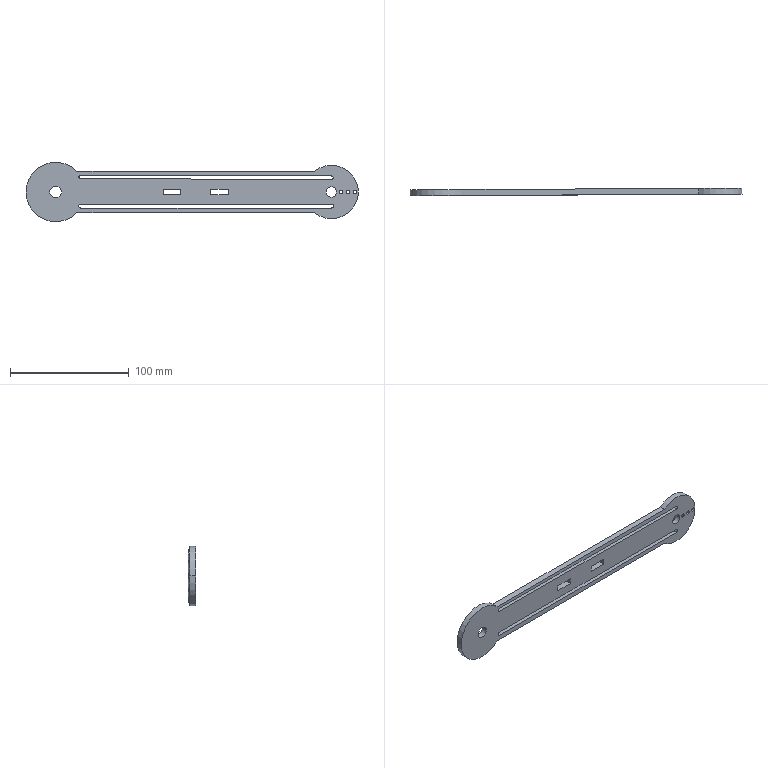Part | SolidWorks | features ICE 3, Extrusion 1 | 1 solid | 35 faces | box 279.515 x 6.264 x 50 mm | volume 42669 mm3 | cylinder 19 | plane 16 | commonest cylinder face diameters 3 x9 3.268 x3 8.5 x2 10 x2 50 x2 45 x1
STEP:
#1=CARTESIAN_POINT('',(-111.192,316.68,396.082));
#2=VERTEX_POINT('',#1);
#3=CARTESIAN_POINT('',(-112.826,316.673,394.448));
#4=VERTEX_POINT('',#3);
#5=CARTESIAN_POINT('',(-111.192,316.68,394.448));
#6=DIRECTION('',(0.004524,-1.,0.));
#7=DIRECTION('',(1.,0.004524,0.));
#8=AXIS2_PLACEMENT_3D('',#5,#6,#7);
#9=CIRCLE('',#8,1.634);
#10=EDGE_CURVE('',#2,#4,#9,.T.);
#11=ORIENTED_EDGE('',*,*,#10,.T.);
#12=CARTESIAN_POINT('',(-112.848,321.673,394.448));
#13=VERTEX_POINT('',#12);
#14=CARTESIAN_POINT('',(-112.803,311.673,394.448));
#15=DIRECTION('',(-0.004524,1.,0.));
#16=VECTOR('',#15,1000.);
#17=LINE('',#14,#16);
#18=EDGE_CURVE('',#4,#13,#17,.T.);
#19=ORIENTED_EDGE('',*,*,#18,.T.);
#20=CARTESIAN_POINT('',(-111.214,321.68,396.082));
#21=VERTEX_POINT('',#20);
#22=CARTESIAN_POINT('',(-111.214,321.68,394.448));
#23=DIRECTION('',(-0.004524,1.,0.));
#24=DIRECTION('',(-1.,-0.004524,0.));
#25=AXIS2_PLACEMENT_3D('',#22,#23,#24);
#26=CIRCLE('',#25,1.634);
#27=EDGE_CURVE('',#13,#21,#26,.T.);
#28=ORIENTED_EDGE('',*,*,#27,.T.);
#29=CARTESIAN_POINT('',(-111.169,311.68,396.082));
#30=DIRECTION('',(-0.004524,1.,0.));
#31=VECTOR('',#30,1000.);
#32=LINE('',#29,#31);
#33=EDGE_CURVE('',#2,#21,#32,.T.);
#34=ORIENTED_EDGE('',*,*,#33,.F.);
#35=EDGE_LOOP('',(#11,#19,#28,#34));
#36=FACE_OUTER_BOUND('',#35,.T.);
#37=CARTESIAN_POINT('',(-111.169,311.68,394.448));
#38=DIRECTION('',(-0.004524,1.,0.));
#39=DIRECTION('',(-1.,-0.004524,0.));
#40=AXIS2_PLACEMENT_3D('',#37,#38,#39);
#41=CYLINDRICAL_SURFACE('',#40,1.634);
#42=ADVANCED_FACE('',(#36),#41,.F.);
#43=CARTESIAN_POINT('',(-111.186,316.68,420.593));
#44=VERTEX_POINT('',#43);
#45=CARTESIAN_POINT('',(-112.692,316.673,419.093));
#46=VERTEX_POINT('',#45);
#47=CARTESIAN_POINT('',(-111.192,316.68,419.093));
#48=DIRECTION('',(0.004524,-1.,0.));
#49=DIRECTION('',(1.,0.004524,0.));
#50=AXIS2_PLACEMENT_3D('',#47,#48,#49);
#51=CIRCLE('',#50,1.5);
#52=EDGE_CURVE('',#44,#46,#51,.T.);
#53=ORIENTED_EDGE('',*,*,#52,.T.);
#54=CARTESIAN_POINT('',(-112.714,321.673,419.093));
#55=VERTEX_POINT('',#54);
#56=CARTESIAN_POINT('',(-112.669,311.673,419.093));
#57=DIRECTION('',(-0.004524,1.,0.));
#58=VECTOR('',#57,1000.);
#59=LINE('',#56,#58);
#60=EDGE_CURVE('',#46,#55,#59,.T.);
#61=ORIENTED_EDGE('',*,*,#60,.T.);
#62=CARTESIAN_POINT('',(-111.209,321.68,420.593));
#63=VERTEX_POINT('',#62);
#64=CARTESIAN_POINT('',(-111.214,321.68,419.093));
#65=DIRECTION('',(-0.004524,1.,0.));
#66=DIRECTION('',(1.,0.004524,0.));
#67=AXIS2_PLACEMENT_3D('',#64,#65,#66);
#68=CIRCLE('',#67,1.5);
#69=EDGE_CURVE('',#55,#63,#68,.T.);
#70=ORIENTED_EDGE('',*,*,#69,.T.);
#71=CARTESIAN_POINT('',(-111.164,311.68,420.593));
#72=DIRECTION('',(-0.004524,1.,0.));
#73=VECTOR('',#72,1000.);
#74=LINE('',#71,#73);
#75=EDGE_CURVE('',#44,#63,#74,.T.);
#76=ORIENTED_EDGE('',*,*,#75,.F.);
#77=EDGE_LOOP('',(#53,#61,#70,#76));
#78=FACE_OUTER_BOUND('',#77,.T.);
#79=CARTESIAN_POINT('',(-111.169,311.68,419.093));
#80=DIRECTION('',(-0.004524,1.,0.));
#81=DIRECTION('',(-1.,-0.004524,0.));
#82=AXIS2_PLACEMENT_3D('',#79,#80,#81);
#83=CYLINDRICAL_SURFACE('',#82,1.5);
#84=ADVANCED_FACE('',(#78),#83,.F.);
#85=CARTESIAN_POINT('',(106.283,317.664,406.314));
#86=VERTEX_POINT('',#85);
#87=CARTESIAN_POINT('',(109.283,317.678,406.314));
#88=VERTEX_POINT('',#87);
#89=CARTESIAN_POINT('',(107.783,317.671,406.314));
#90=DIRECTION('',(0.004524,-1.,0.));
#91=DIRECTION('',(1.,0.004524,0.));
#92=AXIS2_PLACEMENT_3D('',#89,#90,#91);
#93=CIRCLE('',#92,1.5);
#94=EDGE_CURVE('',#86,#88,#93,.T.);
#95=ORIENTED_EDGE('',*,*,#94,.T.);
#96=CARTESIAN_POINT('',(109.261,322.678,406.314));
#97=VERTEX_POINT('',#96);
#98=CARTESIAN_POINT('',(109.306,312.678,406.314));
#99=DIRECTION('',(-0.004524,1.,0.));
#100=VECTOR('',#99,1000.);
#101=LINE('',#98,#100);
#102=EDGE_CURVE('',#88,#97,#101,.T.);
#103=ORIENTED_EDGE('',*,*,#102,.T.);
#104=CARTESIAN_POINT('',(106.261,322.664,406.314));
#105=VERTEX_POINT('',#104);
#106=CARTESIAN_POINT('',(107.761,322.671,406.314));
#107=DIRECTION('',(-0.004524,1.,0.));
#108=DIRECTION('',(-1.,-0.004524,0.));
#109=AXIS2_PLACEMENT_3D('',#106,#107,#108);
#110=CIRCLE('',#109,1.5);
#111=EDGE_CURVE('',#97,#105,#110,.T.);
#112=ORIENTED_EDGE('',*,*,#111,.T.);
#113=CARTESIAN_POINT('',(106.306,312.664,406.314));
#114=DIRECTION('',(-0.004524,1.,0.));
#115=VECTOR('',#114,1000.);
#116=LINE('',#113,#115);
#117=EDGE_CURVE('',#86,#105,#116,.T.);
#118=ORIENTED_EDGE('',*,*,#117,.F.);
#119=EDGE_LOOP('',(#95,#103,#112,#118));
#120=FACE_OUTER_BOUND('',#119,.T.);
#121=CARTESIAN_POINT('',(107.806,312.671,406.314));
#122=DIRECTION('',(-0.004524,1.,0.));
#123=DIRECTION('',(-1.,-0.004524,0.));
#124=AXIS2_PLACEMENT_3D('',#121,#122,#123);
#125=CYLINDRICAL_SURFACE('',#124,1.5);
#126=ADVANCED_FACE('',(#120),#125,.F.);
#127=CARTESIAN_POINT('',(112.283,317.691,406.314));
#128=VERTEX_POINT('',#127);
#129=CARTESIAN_POINT('',(115.283,317.705,406.314));
#130=VERTEX_POINT('',#129);
#131=CARTESIAN_POINT('',(113.783,317.698,406.314));
#132=DIRECTION('',(0.004524,-1.,0.));
#133=DIRECTION('',(1.,0.004524,0.));
#134=AXIS2_PLACEMENT_3D('',#131,#132,#133);
#135=CIRCLE('',#134,1.5);
#136=EDGE_CURVE('',#128,#130,#135,.T.);
#137=ORIENTED_EDGE('',*,*,#136,.T.);
#138=CARTESIAN_POINT('',(115.261,322.705,406.314));
#139=VERTEX_POINT('',#138);
#140=CARTESIAN_POINT('',(115.306,312.705,406.314));
#141=DIRECTION('',(-0.004524,1.,0.));
#142=VECTOR('',#141,1000.);
#143=LINE('',#140,#142);
#144=EDGE_CURVE('',#130,#139,#143,.T.);
#145=ORIENTED_EDGE('',*,*,#144,.T.);
#146=CARTESIAN_POINT('',(112.261,322.691,406.314));
#147=VERTEX_POINT('',#146);
#148=CARTESIAN_POINT('',(113.761,322.698,406.314));
#149=DIRECTION('',(-0.004524,1.,0.));
#150=DIRECTION('',(-1.,-0.004524,0.));
#151=AXIS2_PLACEMENT_3D('',#148,#149,#150);
#152=CIRCLE('',#151,1.5);
#153=EDGE_CURVE('',#139,#147,#152,.T.);
#154=ORIENTED_EDGE('',*,*,#153,.T.);
#155=CARTESIAN_POINT('',(112.306,312.691,406.314));
#156=DIRECTION('',(-0.004524,1.,0.));
#157=VECTOR('',#156,1000.);
#158=LINE('',#155,#157);
#159=EDGE_CURVE('',#128,#147,#158,.T.);
#160=ORIENTED_EDGE('',*,*,#159,.F.);
#161=EDGE_LOOP('',(#137,#145,#154,#160));
#162=FACE_OUTER_BOUND('',#161,.T.);
#163=CARTESIAN_POINT('',(113.806,312.698,406.314));
#164=DIRECTION('',(-0.004524,1.,0.));
#165=DIRECTION('',(-1.,-0.004524,0.));
#166=AXIS2_PLACEMENT_3D('',#163,#164,#165);
#167=CYLINDRICAL_SURFACE('',#166,1.5);
#168=ADVANCED_FACE('',(#162),#167,.F.);
#169=CARTESIAN_POINT('',(118.283,317.718,406.314));
#170=VERTEX_POINT('',#169);
#171=CARTESIAN_POINT('',(121.283,317.732,406.314));
#172=VERTEX_POINT('',#171);
#173=CARTESIAN_POINT('',(119.783,317.725,406.314));
#174=DIRECTION('',(0.004524,-1.,0.));
#175=DIRECTION('',(1.,0.004524,0.));
#176=AXIS2_PLACEMENT_3D('',#173,#174,#175);
#177=CIRCLE('',#176,1.5);
#178=EDGE_CURVE('',#170,#172,#177,.T.);
#179=ORIENTED_EDGE('',*,*,#178,.T.);
#180=CARTESIAN_POINT('',(121.261,322.732,406.314));
#181=VERTEX_POINT('',#180);
#182=CARTESIAN_POINT('',(121.306,312.732,406.314));
#183=DIRECTION('',(-0.004524,1.,0.));
#184=VECTOR('',#183,1000.);
#185=LINE('',#182,#184);
#186=EDGE_CURVE('',#172,#181,#185,.T.);
#187=ORIENTED_EDGE('',*,*,#186,.T.);
#188=CARTESIAN_POINT('',(118.261,322.718,406.314));
#189=VERTEX_POINT('',#188);
#190=CARTESIAN_POINT('',(119.761,322.725,406.314));
#191=DIRECTION('',(-0.004524,1.,0.));
#192=DIRECTION('',(-1.,-0.004524,0.));
#193=AXIS2_PLACEMENT_3D('',#190,#191,#192);
#194=CIRCLE('',#193,1.5);
#195=EDGE_CURVE('',#181,#189,#194,.T.);
#196=ORIENTED_EDGE('',*,*,#195,.T.);
#197=CARTESIAN_POINT('',(118.306,312.718,406.314));
#198=DIRECTION('',(-0.004524,1.,0.));
#199=VECTOR('',#198,1000.);
#200=LINE('',#197,#199);
#201=EDGE_CURVE('',#170,#189,#200,.T.);
#202=ORIENTED_EDGE('',*,*,#201,.F.);
#203=EDGE_LOOP('',(#179,#187,#196,#202));
#204=FACE_OUTER_BOUND('',#203,.T.);
#205=CARTESIAN_POINT('',(119.806,312.725,406.314));
#206=DIRECTION('',(-0.004524,1.,0.));
#207=DIRECTION('',(-1.,-0.004524,0.));
#208=AXIS2_PLACEMENT_3D('',#205,#206,#207);
#209=CYLINDRICAL_SURFACE('',#208,1.5);
#210=ADVANCED_FACE('',(#204),#209,.F.);
#211=CARTESIAN_POINT('',(-137.21,316.562,406.314));
#212=VERTEX_POINT('',#211);
#213=CARTESIAN_POINT('',(-127.21,316.608,406.314));
#214=VERTEX_POINT('',#213);
#215=CARTESIAN_POINT('',(-132.21,316.585,406.314));
#216=DIRECTION('',(0.004524,-1.,0.));
#217=DIRECTION('',(1.,0.004524,0.));
#218=AXIS2_PLACEMENT_3D('',#215,#216,#217);
#219=CIRCLE('',#218,5.);
#220=EDGE_CURVE('',#212,#214,#219,.T.);
#221=ORIENTED_EDGE('',*,*,#220,.T.);
#222=CARTESIAN_POINT('',(-127.233,321.608,406.314));
#223=VERTEX_POINT('',#222);
#224=CARTESIAN_POINT('',(-127.21,316.608,406.314));
#225=DIRECTION('',(-0.004524,1.,0.));
#226=VECTOR('',#225,1000.);
#227=LINE('',#224,#226);
#228=EDGE_CURVE('',#214,#223,#227,.T.);
#229=ORIENTED_EDGE('',*,*,#228,.T.);
#230=CARTESIAN_POINT('',(-137.232,321.562,406.314));
#231=VERTEX_POINT('',#230);
#232=CARTESIAN_POINT('',(-132.233,321.585,406.314));
#233=DIRECTION('',(0.004524,-1.,0.));
#234=DIRECTION('',(1.,0.004524,0.));
#235=AXIS2_PLACEMENT_3D('',#232,#233,#234);
#236=CIRCLE('',#235,5.);
#237=EDGE_CURVE('',#231,#223,#236,.T.);
#238=ORIENTED_EDGE('',*,*,#237,.F.);
#239=CARTESIAN_POINT('',(-137.21,316.562,406.314));
#240=DIRECTION('',(-0.004524,1.,0.));
#241=VECTOR('',#240,1000.);
#242=LINE('',#239,#241);
#243=EDGE_CURVE('',#212,#231,#242,.T.);
#244=ORIENTED_EDGE('',*,*,#243,.F.);
#245=EDGE_LOOP('',(#221,#229,#238,#244));
#246=FACE_OUTER_BOUND('',#245,.T.);
#247=CARTESIAN_POINT('',(-132.21,316.585,406.314));
#248=DIRECTION('',(-0.004524,1.,0.));
#249=DIRECTION('',(-1.,-0.004524,0.));
#250=AXIS2_PLACEMENT_3D('',#247,#248,#249);
#251=CYLINDRICAL_SURFACE('',#250,5.);
#252=ADVANCED_FACE('',(#246),#251,.F.);
#253=CARTESIAN_POINT('',(95.533,317.615,406.314));
#254=VERTEX_POINT('',#253);
#255=CARTESIAN_POINT('',(104.033,317.654,406.314));
#256=VERTEX_POINT('',#255);
#257=CARTESIAN_POINT('',(99.783,317.635,406.314));
#258=DIRECTION('',(0.004524,-1.,0.));
#259=DIRECTION('',(1.,0.004524,0.));
#260=AXIS2_PLACEMENT_3D('',#257,#258,#259);
#261=CIRCLE('',#260,4.25);
#262=EDGE_CURVE('',#254,#256,#261,.T.);
#263=ORIENTED_EDGE('',*,*,#262,.T.);
#264=CARTESIAN_POINT('',(104.011,322.654,406.314));
#265=VERTEX_POINT('',#264);
#266=CARTESIAN_POINT('',(104.033,317.654,406.314));
#267=DIRECTION('',(-0.004524,1.,0.));
#268=VECTOR('',#267,1000.);
#269=LINE('',#266,#268);
#270=EDGE_CURVE('',#256,#265,#269,.T.);
#271=ORIENTED_EDGE('',*,*,#270,.T.);
#272=CARTESIAN_POINT('',(95.511,322.615,406.314));
#273=VERTEX_POINT('',#272);
#274=CARTESIAN_POINT('',(99.761,322.635,406.314));
#275=DIRECTION('',(0.004524,-1.,0.));
#276=DIRECTION('',(1.,0.004524,0.));
#277=AXIS2_PLACEMENT_3D('',#274,#275,#276);
#278=CIRCLE('',#277,4.25);
#279=EDGE_CURVE('',#273,#265,#278,.T.);
#280=ORIENTED_EDGE('',*,*,#279,.F.);
#281=CARTESIAN_POINT('',(95.533,317.615,406.314));
#282=DIRECTION('',(-0.004524,1.,0.));
#283=VECTOR('',#282,1000.);
#284=LINE('',#281,#283);
#285=EDGE_CURVE('',#254,#273,#284,.T.);
#286=ORIENTED_EDGE('',*,*,#285,.F.);
#287=EDGE_LOOP('',(#263,#271,#280,#286));
#288=FACE_OUTER_BOUND('',#287,.T.);
#289=CARTESIAN_POINT('',(99.783,317.635,406.314));
#290=DIRECTION('',(-0.004524,1.,0.));
#291=DIRECTION('',(-1.,-0.004524,0.));
#292=AXIS2_PLACEMENT_3D('',#289,#290,#291);
#293=CYLINDRICAL_SURFACE('',#292,4.25);
#294=ADVANCED_FACE('',(#288),#293,.F.);
#295=CARTESIAN_POINT('',(-157.21,316.472,406.314));
#296=VERTEX_POINT('',#295);
#297=CARTESIAN_POINT('',(-114.357,316.666,388.814));
#298=VERTEX_POINT('',#297);
#299=CARTESIAN_POINT('',(-132.21,316.585,406.314));
#300=DIRECTION('',(0.004524,-1.,0.));
#301=DIRECTION('',(1.,0.004524,0.));
#302=AXIS2_PLACEMENT_3D('',#299,#300,#301);
#303=CIRCLE('',#302,25.);
#304=EDGE_CURVE('',#296,#298,#303,.T.);
#305=ORIENTED_EDGE('',*,*,#304,.F.);
#306=CARTESIAN_POINT('',(-157.232,321.472,406.314));
#307=VERTEX_POINT('',#306);
#308=CARTESIAN_POINT('',(-157.21,316.472,406.314));
#309=DIRECTION('',(-0.004524,1.,0.));
#310=VECTOR('',#309,1000.);
#311=LINE('',#308,#310);
#312=EDGE_CURVE('',#296,#307,#311,.T.);
#313=ORIENTED_EDGE('',*,*,#312,.T.);
#314=CARTESIAN_POINT('',(-114.379,321.666,388.814));
#315=VERTEX_POINT('',#314);
#316=CARTESIAN_POINT('',(-132.233,321.585,406.314));
#317=DIRECTION('',(0.004524,-1.,0.));
#318=DIRECTION('',(1.,0.004524,0.));
#319=AXIS2_PLACEMENT_3D('',#316,#317,#318);
#320=CIRCLE('',#319,25.);
#321=EDGE_CURVE('',#307,#315,#320,.T.);
#322=ORIENTED_EDGE('',*,*,#321,.T.);
#323=CARTESIAN_POINT('',(-114.357,316.666,388.814));
#324=DIRECTION('',(-0.004524,1.,0.));
#325=VECTOR('',#324,1000.);
#326=LINE('',#323,#325);
#327=EDGE_CURVE('',#298,#315,#326,.T.);
#328=ORIENTED_EDGE('',*,*,#327,.F.);
#329=EDGE_LOOP('',(#305,#313,#322,#328));
#330=FACE_OUTER_BOUND('',#329,.T.);
#331=CARTESIAN_POINT('',(-132.21,316.585,406.314));
#332=DIRECTION('',(-0.004524,1.,0.));
#333=DIRECTION('',(-1.,-0.004524,0.));
#334=AXIS2_PLACEMENT_3D('',#331,#332,#333);
#335=CYLINDRICAL_SURFACE('',#334,25.);
#336=ADVANCED_FACE('',(#330),#335,.T.);
#337=CARTESIAN_POINT('',(-41.857,316.994,408.814));
#338=VERTEX_POINT('',#337);
#339=CARTESIAN_POINT('',(-41.857,316.994,403.814));
#340=VERTEX_POINT('',#339);
#341=CARTESIAN_POINT('',(-41.857,316.994,406.314));
#342=DIRECTION('',(0.,0.,-1.));
#343=VECTOR('',#342,1000.);
#344=LINE('',#341,#343);
#345=EDGE_CURVE('',#338,#340,#344,.T.);
#346=ORIENTED_EDGE('',*,*,#345,.F.);
#347=CARTESIAN_POINT('',(-26.857,317.062,408.814));
#348=VERTEX_POINT('',#347);
#349=CARTESIAN_POINT('',(99.783,317.635,408.814));
#350=DIRECTION('',(-1.,-0.004524,0.));
#351=VECTOR('',#350,1000.);
#352=LINE('',#349,#351);
#353=EDGE_CURVE('',#348,#338,#352,.T.);
#354=ORIENTED_EDGE('',*,*,#353,.F.);
#355=CARTESIAN_POINT('',(-26.857,317.062,403.814));
#356=VERTEX_POINT('',#355);
#357=CARTESIAN_POINT('',(-26.857,317.062,406.314));
#358=DIRECTION('',(0.,0.,1.));
#359=VECTOR('',#358,1000.);
#360=LINE('',#357,#359);
#361=EDGE_CURVE('',#356,#348,#360,.T.);
#362=ORIENTED_EDGE('',*,*,#361,.F.);
#363=CARTESIAN_POINT('',(99.783,317.635,403.814));
#364=DIRECTION('',(1.,0.004524,0.));
#365=VECTOR('',#364,1000.);
#366=LINE('',#363,#365);
#367=EDGE_CURVE('',#340,#356,#366,.T.);
#368=ORIENTED_EDGE('',*,*,#367,.F.);
#369=EDGE_LOOP('',(#346,#354,#362,#368));
#370=FACE_BOUND('',#369,.T.);
#371=CARTESIAN_POINT('',(-1.858,317.175,408.814));
#372=VERTEX_POINT('',#371);
#373=CARTESIAN_POINT('',(-1.858,317.175,403.814));
#374=VERTEX_POINT('',#373);
#375=CARTESIAN_POINT('',(-1.858,317.175,406.314));
#376=DIRECTION('',(0.,0.,-1.));
#377=VECTOR('',#376,1000.);
#378=LINE('',#375,#377);
#379=EDGE_CURVE('',#372,#374,#378,.T.);
#380=ORIENTED_EDGE('',*,*,#379,.F.);
#381=CARTESIAN_POINT('',(13.142,317.243,408.814));
#382=VERTEX_POINT('',#381);
#383=CARTESIAN_POINT('',(99.783,317.635,408.814));
#384=DIRECTION('',(-1.,-0.004524,0.));
#385=VECTOR('',#384,1000.);
#386=LINE('',#383,#385);
#387=EDGE_CURVE('',#382,#372,#386,.T.);
#388=ORIENTED_EDGE('',*,*,#387,.F.);
#389=CARTESIAN_POINT('',(13.142,317.243,403.814));
#390=VERTEX_POINT('',#389);
#391=CARTESIAN_POINT('',(13.142,317.243,406.314));
#392=DIRECTION('',(0.,0.,1.));
#393=VECTOR('',#392,1000.);
#394=LINE('',#391,#393);
#395=EDGE_CURVE('',#390,#382,#394,.T.);
#396=ORIENTED_EDGE('',*,*,#395,.F.);
#397=CARTESIAN_POINT('',(99.783,317.635,403.814));
#398=DIRECTION('',(1.,0.004524,0.));
#399=VECTOR('',#398,1000.);
#400=LINE('',#397,#399);
#401=EDGE_CURVE('',#374,#390,#400,.T.);
#402=ORIENTED_EDGE('',*,*,#401,.F.);
#403=EDGE_LOOP('',(#380,#388,#396,#402));
#404=FACE_BOUND('',#403,.T.);
#405=ORIENTED_EDGE('',*,*,#10,.F.);
#406=CARTESIAN_POINT('',(99.783,317.635,396.082));
#407=VERTEX_POINT('',#406);
#408=CARTESIAN_POINT('',(99.783,317.635,396.082));
#409=DIRECTION('',(-1.,-0.004524,0.));
#410=VECTOR('',#409,1000.);
#411=LINE('',#408,#410);
#412=EDGE_CURVE('',#407,#2,#411,.T.);
#413=ORIENTED_EDGE('',*,*,#412,.F.);
#414=CARTESIAN_POINT('',(99.783,317.635,392.814));
#415=VERTEX_POINT('',#414);
#416=CARTESIAN_POINT('',(99.783,317.635,394.448));
#417=DIRECTION('',(0.004524,-1.,0.));
#418=DIRECTION('',(1.,0.004524,0.));
#419=AXIS2_PLACEMENT_3D('',#416,#417,#418);
#420=CIRCLE('',#419,1.634);
#421=EDGE_CURVE('',#415,#407,#420,.T.);
#422=ORIENTED_EDGE('',*,*,#421,.F.);
#423=CARTESIAN_POINT('',(-111.192,316.68,392.814));
#424=VERTEX_POINT('',#423);
#425=CARTESIAN_POINT('',(99.783,317.635,392.814));
#426=DIRECTION('',(1.,0.004524,0.));
#427=VECTOR('',#426,1000.);
#428=LINE('',#425,#427);
#429=EDGE_CURVE('',#424,#415,#428,.T.);
#430=ORIENTED_EDGE('',*,*,#429,.F.);
#431=CARTESIAN_POINT('',(-111.192,316.68,394.448));
#432=DIRECTION('',(0.004524,-1.,0.));
#433=DIRECTION('',(1.,0.004524,0.));
#434=AXIS2_PLACEMENT_3D('',#431,#432,#433);
#435=CIRCLE('',#434,1.634);
#436=EDGE_CURVE('',#4,#424,#435,.T.);
#437=ORIENTED_EDGE('',*,*,#436,.F.);
#438=EDGE_LOOP('',(#405,#413,#422,#430,#437));
#439=FACE_BOUND('',#438,.T.);
#440=ORIENTED_EDGE('',*,*,#52,.F.);
#441=CARTESIAN_POINT('',(99.783,317.635,419.814));
#442=VERTEX_POINT('',#441);
#443=CARTESIAN_POINT('',(99.833,317.635,419.814));
#444=DIRECTION('',(-1.,-0.004524,0.003693));
#445=VECTOR('',#444,1000.);
#446=LINE('',#443,#445);
#447=EDGE_CURVE('',#442,#44,#446,.T.);
#448=ORIENTED_EDGE('',*,*,#447,.F.);
#449=CARTESIAN_POINT('',(99.772,317.635,416.814));
#450=VERTEX_POINT('',#449);
#451=CARTESIAN_POINT('',(99.778,317.635,418.314));
#452=DIRECTION('',(0.004524,-1.,0.));
#453=DIRECTION('',(1.,0.004524,0.));
#454=AXIS2_PLACEMENT_3D('',#451,#452,#453);
#455=CIRCLE('',#454,1.5);
#456=EDGE_CURVE('',#450,#442,#455,.T.);
#457=ORIENTED_EDGE('',*,*,#456,.F.);
#458=CARTESIAN_POINT('',(-111.197,316.68,417.593));
#459=VERTEX_POINT('',#458);
#460=CARTESIAN_POINT('',(99.822,317.635,416.814));
#461=DIRECTION('',(1.,0.004524,-0.003693));
#462=VECTOR('',#461,1000.);
#463=LINE('',#460,#462);
#464=EDGE_CURVE('',#459,#450,#463,.T.);
#465=ORIENTED_EDGE('',*,*,#464,.F.);
#466=CARTESIAN_POINT('',(-111.192,316.68,419.093));
#467=DIRECTION('',(0.004524,-1.,0.));
#468=DIRECTION('',(1.,0.004524,0.));
#469=AXIS2_PLACEMENT_3D('',#466,#467,#468);
#470=CIRCLE('',#469,1.5);
#471=EDGE_CURVE('',#46,#459,#470,.T.);
#472=ORIENTED_EDGE('',*,*,#471,.F.);
#473=EDGE_LOOP('',(#440,#448,#457,#465,#472));
#474=FACE_BOUND('',#473,.T.);
#475=ORIENTED_EDGE('',*,*,#94,.F.);
#476=CARTESIAN_POINT('',(107.783,317.671,406.314));
#477=DIRECTION('',(0.004524,-1.,0.));
#478=DIRECTION('',(1.,0.004524,0.));
#479=AXIS2_PLACEMENT_3D('',#476,#477,#478);
#480=CIRCLE('',#479,1.5);
#481=EDGE_CURVE('',#88,#86,#480,.T.);
#482=ORIENTED_EDGE('',*,*,#481,.F.);
#483=EDGE_LOOP('',(#475,#482));
#484=FACE_BOUND('',#483,.T.);
#485=ORIENTED_EDGE('',*,*,#136,.F.);
#486=CARTESIAN_POINT('',(113.783,317.698,406.314));
#487=DIRECTION('',(0.004524,-1.,0.));
#488=DIRECTION('',(1.,0.004524,0.));
#489=AXIS2_PLACEMENT_3D('',#486,#487,#488);
#490=CIRCLE('',#489,1.5);
#491=EDGE_CURVE('',#130,#128,#490,.T.);
#492=ORIENTED_EDGE('',*,*,#491,.F.);
#493=EDGE_LOOP('',(#485,#492));
#494=FACE_BOUND('',#493,.T.);
#495=ORIENTED_EDGE('',*,*,#178,.F.);
#496=CARTESIAN_POINT('',(119.783,317.725,406.314));
#497=DIRECTION('',(0.004524,-1.,0.));
#498=DIRECTION('',(1.,0.004524,0.));
#499=AXIS2_PLACEMENT_3D('',#496,#497,#498);
#500=CIRCLE('',#499,1.5);
#501=EDGE_CURVE('',#172,#170,#500,.T.);
#502=ORIENTED_EDGE('',*,*,#501,.F.);
#503=EDGE_LOOP('',(#495,#502));
#504=FACE_BOUND('',#503,.T.);
#505=ORIENTED_EDGE('',*,*,#262,.F.);
#506=CARTESIAN_POINT('',(99.783,317.635,406.314));
#507=DIRECTION('',(0.004524,-1.,0.));
#508=DIRECTION('',(1.,0.004524,0.));
#509=AXIS2_PLACEMENT_3D('',#506,#507,#508);
#510=CIRCLE('',#509,4.25);
#511=EDGE_CURVE('',#256,#254,#510,.T.);
#512=ORIENTED_EDGE('',*,*,#511,.F.);
#513=EDGE_LOOP('',(#505,#512));
#514=FACE_BOUND('',#513,.T.);
#515=CARTESIAN_POINT('',(85.641,317.571,388.814));
#516=VERTEX_POINT('',#515);
#517=CARTESIAN_POINT('',(85.641,317.571,423.814));
#518=VERTEX_POINT('',#517);
#519=CARTESIAN_POINT('',(99.783,317.635,406.314));
#520=DIRECTION('',(0.004524,-1.,0.));
#521=DIRECTION('',(1.,0.004524,0.));
#522=AXIS2_PLACEMENT_3D('',#519,#520,#521);
#523=CIRCLE('',#522,22.5);
#524=EDGE_CURVE('',#516,#518,#523,.T.);
#525=ORIENTED_EDGE('',*,*,#524,.T.);
#526=CARTESIAN_POINT('',(-114.357,316.666,423.814));
#527=VERTEX_POINT('',#526);
#528=CARTESIAN_POINT('',(85.641,317.571,423.814));
#529=DIRECTION('',(-1.,-0.004524,0.));
#530=VECTOR('',#529,1000.);
#531=LINE('',#528,#530);
#532=EDGE_CURVE('',#518,#527,#531,.T.);
#533=ORIENTED_EDGE('',*,*,#532,.T.);
#534=CARTESIAN_POINT('',(-132.21,316.585,406.314));
#535=DIRECTION('',(0.004524,-1.,0.));
#536=DIRECTION('',(1.,0.004524,0.));
#537=AXIS2_PLACEMENT_3D('',#534,#535,#536);
#538=CIRCLE('',#537,25.);
#539=EDGE_CURVE('',#527,#296,#538,.T.);
#540=ORIENTED_EDGE('',*,*,#539,.T.);
#541=ORIENTED_EDGE('',*,*,#304,.T.);
#542=CARTESIAN_POINT('',(85.641,317.571,388.814));
#543=DIRECTION('',(1.,0.004524,0.));
#544=VECTOR('',#543,1000.);
#545=LINE('',#542,#544);
#546=EDGE_CURVE('',#298,#516,#545,.T.);
#547=ORIENTED_EDGE('',*,*,#546,.T.);
#548=EDGE_LOOP('',(#525,#533,#540,#541,#547));
#549=FACE_OUTER_BOUND('',#548,.T.);
#550=ORIENTED_EDGE('',*,*,#220,.F.);
#551=CARTESIAN_POINT('',(-132.21,316.585,406.314));
#552=DIRECTION('',(0.004524,-1.,0.));
#553=DIRECTION('',(1.,0.004524,0.));
#554=AXIS2_PLACEMENT_3D('',#551,#552,#553);
#555=CIRCLE('',#554,5.);
#556=EDGE_CURVE('',#214,#212,#555,.T.);
#557=ORIENTED_EDGE('',*,*,#556,.F.);
#558=EDGE_LOOP('',(#550,#557));
#559=FACE_BOUND('',#558,.T.);
#560=CARTESIAN_POINT('',(99.783,317.635,406.314));
#561=DIRECTION('',(0.004524,-1.,0.));
#562=DIRECTION('',(1.,0.004524,0.));
#563=AXIS2_PLACEMENT_3D('',#560,#561,#562);
#564=PLANE('',#563);
#565=ADVANCED_FACE('',(#370,#404,#439,#474,#484,#494,#504,#514,#549,#559),#564,.T.);
#566=CARTESIAN_POINT('',(-41.88,321.994,408.814));
#567=VERTEX_POINT('',#566);
#568=CARTESIAN_POINT('',(-26.88,322.062,408.814));
#569=VERTEX_POINT('',#568);
#570=CARTESIAN_POINT('',(-41.88,321.994,408.814));
#571=DIRECTION('',(1.,0.004524,0.));
#572=VECTOR('',#571,1000.);
#573=LINE('',#570,#572);
#574=EDGE_CURVE('',#567,#569,#573,.T.);
#575=ORIENTED_EDGE('',*,*,#574,.F.);
#576=CARTESIAN_POINT('',(-41.88,321.994,403.814));
#577=VERTEX_POINT('',#576);
#578=CARTESIAN_POINT('',(-41.88,321.994,408.814));
#579=DIRECTION('',(0.,0.,1.));
#580=VECTOR('',#579,1000.);
#581=LINE('',#578,#580);
#582=EDGE_CURVE('',#577,#567,#581,.T.);
#583=ORIENTED_EDGE('',*,*,#582,.F.);
#584=CARTESIAN_POINT('',(-26.88,322.062,403.814));
#585=VERTEX_POINT('',#584);
#586=CARTESIAN_POINT('',(-41.88,321.994,403.814));
#587=DIRECTION('',(-1.,-0.004524,0.));
#588=VECTOR('',#587,1000.);
#589=LINE('',#586,#588);
#590=EDGE_CURVE('',#585,#577,#589,.T.);
#591=ORIENTED_EDGE('',*,*,#590,.F.);
#592=CARTESIAN_POINT('',(-26.88,322.062,408.814));
#593=DIRECTION('',(0.,0.,-1.));
#594=VECTOR('',#593,1000.);
#595=LINE('',#592,#594);
#596=EDGE_CURVE('',#569,#585,#595,.T.);
#597=ORIENTED_EDGE('',*,*,#596,.F.);
#598=EDGE_LOOP('',(#575,#583,#591,#597));
#599=FACE_BOUND('',#598,.T.);
#600=CARTESIAN_POINT('',(-1.88,322.175,408.814));
#601=VERTEX_POINT('',#600);
#602=CARTESIAN_POINT('',(13.12,322.243,408.814));
#603=VERTEX_POINT('',#602);
#604=CARTESIAN_POINT('',(-1.88,322.175,408.814));
#605=DIRECTION('',(1.,0.004524,0.));
#606=VECTOR('',#605,1000.);
#607=LINE('',#604,#606);
#608=EDGE_CURVE('',#601,#603,#607,.T.);
#609=ORIENTED_EDGE('',*,*,#608,.F.);
#610=CARTESIAN_POINT('',(-1.88,322.175,403.814));
#611=VERTEX_POINT('',#610);
#612=CARTESIAN_POINT('',(-1.88,322.175,408.814));
#613=DIRECTION('',(0.,0.,1.));
#614=VECTOR('',#613,1000.);
#615=LINE('',#612,#614);
#616=EDGE_CURVE('',#611,#601,#615,.T.);
#617=ORIENTED_EDGE('',*,*,#616,.F.);
#618=CARTESIAN_POINT('',(13.12,322.243,403.814));
#619=VERTEX_POINT('',#618);
#620=CARTESIAN_POINT('',(-1.88,322.175,403.814));
#621=DIRECTION('',(-1.,-0.004524,0.));
#622=VECTOR('',#621,1000.);
#623=LINE('',#620,#622);
#624=EDGE_CURVE('',#619,#611,#623,.T.);
#625=ORIENTED_EDGE('',*,*,#624,.F.);
#626=CARTESIAN_POINT('',(13.12,322.243,408.814));
#627=DIRECTION('',(0.,0.,-1.));
#628=VECTOR('',#627,1000.);
#629=LINE('',#626,#628);
#630=EDGE_CURVE('',#603,#619,#629,.T.);
#631=ORIENTED_EDGE('',*,*,#630,.F.);
#632=EDGE_LOOP('',(#609,#617,#625,#631));
#633=FACE_BOUND('',#632,.T.);
#634=CARTESIAN_POINT('',(99.761,322.635,396.082));
#635=VERTEX_POINT('',#634);
#636=CARTESIAN_POINT('',(-111.214,321.68,396.082));
#637=DIRECTION('',(1.,0.004524,0.));
#638=VECTOR('',#637,1000.);
#639=LINE('',#636,#638);
#640=EDGE_CURVE('',#21,#635,#639,.T.);
#641=ORIENTED_EDGE('',*,*,#640,.F.);
#642=ORIENTED_EDGE('',*,*,#27,.F.);
#643=CARTESIAN_POINT('',(-111.214,321.68,392.814));
#644=VERTEX_POINT('',#643);
#645=CARTESIAN_POINT('',(-111.214,321.68,394.448));
#646=DIRECTION('',(-0.004524,1.,0.));
#647=DIRECTION('',(-1.,-0.004524,0.));
#648=AXIS2_PLACEMENT_3D('',#645,#646,#647);
#649=CIRCLE('',#648,1.634);
#650=EDGE_CURVE('',#644,#13,#649,.T.);
#651=ORIENTED_EDGE('',*,*,#650,.F.);
#652=CARTESIAN_POINT('',(99.761,322.635,392.814));
#653=VERTEX_POINT('',#652);
#654=CARTESIAN_POINT('',(-111.214,321.68,392.814));
#655=DIRECTION('',(-1.,-0.004524,0.));
#656=VECTOR('',#655,1000.);
#657=LINE('',#654,#656);
#658=EDGE_CURVE('',#653,#644,#657,.T.);
#659=ORIENTED_EDGE('',*,*,#658,.F.);
#660=CARTESIAN_POINT('',(99.761,322.635,394.448));
#661=DIRECTION('',(-0.004524,1.,0.));
#662=DIRECTION('',(-1.,-0.004524,0.));
#663=AXIS2_PLACEMENT_3D('',#660,#661,#662);
#664=CIRCLE('',#663,1.634);
#665=EDGE_CURVE('',#635,#653,#664,.T.);
#666=ORIENTED_EDGE('',*,*,#665,.F.);
#667=EDGE_LOOP('',(#641,#642,#651,#659,#666));
#668=FACE_BOUND('',#667,.T.);
#669=CARTESIAN_POINT('',(99.761,322.635,419.814));
#670=VERTEX_POINT('',#669);
#671=CARTESIAN_POINT('',(-111.209,321.68,420.593));
#672=DIRECTION('',(1.,0.004524,-0.003693));
#673=VECTOR('',#672,1000.);
#674=LINE('',#671,#673);
#675=EDGE_CURVE('',#63,#670,#674,.T.);
#676=ORIENTED_EDGE('',*,*,#675,.F.);
#677=ORIENTED_EDGE('',*,*,#69,.F.);
#678=CARTESIAN_POINT('',(-111.22,321.68,417.593));
#679=VERTEX_POINT('',#678);
#680=CARTESIAN_POINT('',(-111.214,321.68,419.093));
#681=DIRECTION('',(-0.004524,1.,0.));
#682=DIRECTION('',(1.,0.004524,0.));
#683=AXIS2_PLACEMENT_3D('',#680,#681,#682);
#684=CIRCLE('',#683,1.5);
#685=EDGE_CURVE('',#679,#55,#684,.T.);
#686=ORIENTED_EDGE('',*,*,#685,.F.);
#687=CARTESIAN_POINT('',(99.75,322.635,416.814));
#688=VERTEX_POINT('',#687);
#689=CARTESIAN_POINT('',(-111.22,321.68,417.593));
#690=DIRECTION('',(-1.,-0.004524,0.003693));
#691=VECTOR('',#690,1000.);
#692=LINE('',#689,#691);
#693=EDGE_CURVE('',#688,#679,#692,.T.);
#694=ORIENTED_EDGE('',*,*,#693,.F.);
#695=CARTESIAN_POINT('',(99.755,322.635,418.314));
#696=DIRECTION('',(-0.004524,1.,0.));
#697=DIRECTION('',(1.,0.004524,0.));
#698=AXIS2_PLACEMENT_3D('',#695,#696,#697);
#699=CIRCLE('',#698,1.5);
#700=EDGE_CURVE('',#670,#688,#699,.T.);
#701=ORIENTED_EDGE('',*,*,#700,.F.);
#702=EDGE_LOOP('',(#676,#677,#686,#694,#701));
#703=FACE_BOUND('',#702,.T.);
#704=CARTESIAN_POINT('',(107.761,322.671,406.314));
#705=DIRECTION('',(-0.004524,1.,0.));
#706=DIRECTION('',(-1.,-0.004524,0.));
#707=AXIS2_PLACEMENT_3D('',#704,#705,#706);
#708=CIRCLE('',#707,1.5);
#709=EDGE_CURVE('',#105,#97,#708,.T.);
#710=ORIENTED_EDGE('',*,*,#709,.F.);
#711=ORIENTED_EDGE('',*,*,#111,.F.);
#712=EDGE_LOOP('',(#710,#711));
#713=FACE_BOUND('',#712,.T.);
#714=CARTESIAN_POINT('',(113.761,322.698,406.314));
#715=DIRECTION('',(-0.004524,1.,0.));
#716=DIRECTION('',(-1.,-0.004524,0.));
#717=AXIS2_PLACEMENT_3D('',#714,#715,#716);
#718=CIRCLE('',#717,1.5);
#719=EDGE_CURVE('',#147,#139,#718,.T.);
#720=ORIENTED_EDGE('',*,*,#719,.F.);
#721=ORIENTED_EDGE('',*,*,#153,.F.);
#722=EDGE_LOOP('',(#720,#721));
#723=FACE_BOUND('',#722,.T.);
#724=CARTESIAN_POINT('',(119.761,322.725,406.314));
#725=DIRECTION('',(-0.004524,1.,0.));
#726=DIRECTION('',(-1.,-0.004524,0.));
#727=AXIS2_PLACEMENT_3D('',#724,#725,#726);
#728=CIRCLE('',#727,1.5);
#729=EDGE_CURVE('',#189,#181,#728,.T.);
#730=ORIENTED_EDGE('',*,*,#729,.F.);
#731=ORIENTED_EDGE('',*,*,#195,.F.);
#732=EDGE_LOOP('',(#730,#731));
#733=FACE_BOUND('',#732,.T.);
#734=CARTESIAN_POINT('',(85.619,322.571,388.814));
#735=VERTEX_POINT('',#734);
#736=CARTESIAN_POINT('',(85.619,322.571,423.814));
#737=VERTEX_POINT('',#736);
#738=CARTESIAN_POINT('',(99.761,322.635,406.314));
#739=DIRECTION('',(0.004524,-1.,0.));
#740=DIRECTION('',(1.,0.004524,0.));
#741=AXIS2_PLACEMENT_3D('',#738,#739,#740);
#742=CIRCLE('',#741,22.5);
#743=EDGE_CURVE('',#735,#737,#742,.T.);
#744=ORIENTED_EDGE('',*,*,#743,.F.);
#745=CARTESIAN_POINT('',(85.619,322.571,388.814));
#746=DIRECTION('',(1.,0.004524,0.));
#747=VECTOR('',#746,1000.);
#748=LINE('',#745,#747);
#749=EDGE_CURVE('',#315,#735,#748,.T.);
#750=ORIENTED_EDGE('',*,*,#749,.F.);
#751=ORIENTED_EDGE('',*,*,#321,.F.);
#752=CARTESIAN_POINT('',(-114.379,321.666,423.814));
#753=VERTEX_POINT('',#752);
#754=CARTESIAN_POINT('',(-132.233,321.585,406.314));
#755=DIRECTION('',(0.004524,-1.,0.));
#756=DIRECTION('',(1.,0.004524,0.));
#757=AXIS2_PLACEMENT_3D('',#754,#755,#756);
#758=CIRCLE('',#757,25.);
#759=EDGE_CURVE('',#753,#307,#758,.T.);
#760=ORIENTED_EDGE('',*,*,#759,.F.);
#761=CARTESIAN_POINT('',(85.619,322.571,423.814));
#762=DIRECTION('',(-1.,-0.004524,0.));
#763=VECTOR('',#762,1000.);
#764=LINE('',#761,#763);
#765=EDGE_CURVE('',#737,#753,#764,.T.);
#766=ORIENTED_EDGE('',*,*,#765,.F.);
#767=EDGE_LOOP('',(#744,#750,#751,#760,#766));
#768=FACE_OUTER_BOUND('',#767,.T.);
#769=ORIENTED_EDGE('',*,*,#279,.T.);
#770=CARTESIAN_POINT('',(99.761,322.635,406.314));
#771=DIRECTION('',(0.004524,-1.,0.));
#772=DIRECTION('',(1.,0.004524,0.));
#773=AXIS2_PLACEMENT_3D('',#770,#771,#772);
#774=CIRCLE('',#773,4.25);
#775=EDGE_CURVE('',#265,#273,#774,.T.);
#776=ORIENTED_EDGE('',*,*,#775,.T.);
#777=EDGE_LOOP('',(#769,#776));
#778=FACE_BOUND('',#777,.T.);
#779=ORIENTED_EDGE('',*,*,#237,.T.);
#780=CARTESIAN_POINT('',(-132.233,321.585,406.314));
#781=DIRECTION('',(0.004524,-1.,0.));
#782=DIRECTION('',(1.,0.004524,0.));
#783=AXIS2_PLACEMENT_3D('',#780,#781,#782);
#784=CIRCLE('',#783,5.);
#785=EDGE_CURVE('',#223,#231,#784,.T.);
#786=ORIENTED_EDGE('',*,*,#785,.T.);
#787=EDGE_LOOP('',(#779,#786));
#788=FACE_BOUND('',#787,.T.);
#789=CARTESIAN_POINT('',(99.761,322.635,406.314));
#790=DIRECTION('',(0.004524,-1.,0.));
#791=DIRECTION('',(1.,0.004524,0.));
#792=AXIS2_PLACEMENT_3D('',#789,#790,#791);
#793=PLANE('',#792);
#794=ADVANCED_FACE('',(#599,#633,#668,#703,#713,#723,#733,#768,#778,#788),#793,.F.);
#795=ORIENTED_EDGE('',*,*,#743,.T.);
#796=CARTESIAN_POINT('',(85.641,317.571,423.814));
#797=DIRECTION('',(-0.004524,1.,0.));
#798=VECTOR('',#797,1000.);
#799=LINE('',#796,#798);
#800=EDGE_CURVE('',#518,#737,#799,.T.);
#801=ORIENTED_EDGE('',*,*,#800,.F.);
#802=ORIENTED_EDGE('',*,*,#524,.F.);
#803=CARTESIAN_POINT('',(85.641,317.571,388.814));
#804=DIRECTION('',(-0.004524,1.,0.));
#805=VECTOR('',#804,1000.);
#806=LINE('',#803,#805);
#807=EDGE_CURVE('',#516,#735,#806,.T.);
#808=ORIENTED_EDGE('',*,*,#807,.T.);
#809=EDGE_LOOP('',(#795,#801,#802,#808));
#810=FACE_OUTER_BOUND('',#809,.T.);
#811=CARTESIAN_POINT('',(99.783,317.635,406.314));
#812=DIRECTION('',(-0.004524,1.,0.));
#813=DIRECTION('',(-1.,-0.004524,0.));
#814=AXIS2_PLACEMENT_3D('',#811,#812,#813);
#815=CYLINDRICAL_SURFACE('',#814,22.5);
#816=ADVANCED_FACE('',(#810),#815,.T.);
#817=ORIENTED_EDGE('',*,*,#765,.T.);
#818=CARTESIAN_POINT('',(-114.357,316.666,423.814));
#819=DIRECTION('',(-0.004524,1.,0.));
#820=VECTOR('',#819,1000.);
#821=LINE('',#818,#820);
#822=EDGE_CURVE('',#527,#753,#821,.T.);
#823=ORIENTED_EDGE('',*,*,#822,.F.);
#824=ORIENTED_EDGE('',*,*,#532,.F.);
#825=ORIENTED_EDGE('',*,*,#800,.T.);
#826=EDGE_LOOP('',(#817,#823,#824,#825));
#827=FACE_OUTER_BOUND('',#826,.T.);
#828=CARTESIAN_POINT('',(85.641,317.571,423.814));
#829=DIRECTION('',(0.,0.,-1.));
#830=DIRECTION('',(-1.,0.,0.));
#831=AXIS2_PLACEMENT_3D('',#828,#829,#830);
#832=PLANE('',#831);
#833=ADVANCED_FACE('',(#827),#832,.F.);
#834=ORIENTED_EDGE('',*,*,#312,.F.);
#835=ORIENTED_EDGE('',*,*,#539,.F.);
#836=ORIENTED_EDGE('',*,*,#822,.T.);
#837=ORIENTED_EDGE('',*,*,#759,.T.);
#838=EDGE_LOOP('',(#834,#835,#836,#837));
#839=FACE_OUTER_BOUND('',#838,.T.);
#840=CARTESIAN_POINT('',(-132.21,316.585,406.314));
#841=DIRECTION('',(-0.004524,1.,0.));
#842=DIRECTION('',(-1.,-0.004524,0.));
#843=AXIS2_PLACEMENT_3D('',#840,#841,#842);
#844=CYLINDRICAL_SURFACE('',#843,25.);
#845=ADVANCED_FACE('',(#839),#844,.T.);
#846=ORIENTED_EDGE('',*,*,#749,.T.);
#847=ORIENTED_EDGE('',*,*,#807,.F.);
#848=ORIENTED_EDGE('',*,*,#546,.F.);
#849=ORIENTED_EDGE('',*,*,#327,.T.);
#850=EDGE_LOOP('',(#846,#847,#848,#849));
#851=FACE_OUTER_BOUND('',#850,.T.);
#852=CARTESIAN_POINT('',(85.641,317.571,388.814));
#853=DIRECTION('',(0.,0.,1.));
#854=DIRECTION('',(0.,-1.,0.));
#855=AXIS2_PLACEMENT_3D('',#852,#853,#854);
#856=PLANE('',#855);
#857=ADVANCED_FACE('',(#851),#856,.F.);
#858=ORIENTED_EDGE('',*,*,#270,.F.);
#859=ORIENTED_EDGE('',*,*,#511,.T.);
#860=ORIENTED_EDGE('',*,*,#285,.T.);
#861=ORIENTED_EDGE('',*,*,#775,.F.);
#862=EDGE_LOOP('',(#858,#859,#860,#861));
#863=FACE_OUTER_BOUND('',#862,.T.);
#864=CARTESIAN_POINT('',(99.783,317.635,406.314));
#865=DIRECTION('',(-0.004524,1.,0.));
#866=DIRECTION('',(-1.,-0.004524,0.));
#867=AXIS2_PLACEMENT_3D('',#864,#865,#866);
#868=CYLINDRICAL_SURFACE('',#867,4.25);
#869=ADVANCED_FACE('',(#863),#868,.F.);
#870=ORIENTED_EDGE('',*,*,#228,.F.);
#871=ORIENTED_EDGE('',*,*,#556,.T.);
#872=ORIENTED_EDGE('',*,*,#243,.T.);
#873=ORIENTED_EDGE('',*,*,#785,.F.);
#874=EDGE_LOOP('',(#870,#871,#872,#873));
#875=FACE_OUTER_BOUND('',#874,.T.);
#876=CARTESIAN_POINT('',(-132.21,316.585,406.314));
#877=DIRECTION('',(-0.004524,1.,0.));
#878=DIRECTION('',(-1.,-0.004524,0.));
#879=AXIS2_PLACEMENT_3D('',#876,#877,#878);
#880=CYLINDRICAL_SURFACE('',#879,5.);
#881=ADVANCED_FACE('',(#875),#880,.F.);
#882=ORIENTED_EDGE('',*,*,#186,.F.);
#883=ORIENTED_EDGE('',*,*,#501,.T.);
#884=ORIENTED_EDGE('',*,*,#201,.T.);
#885=ORIENTED_EDGE('',*,*,#729,.T.);
#886=EDGE_LOOP('',(#882,#883,#884,#885));
#887=FACE_OUTER_BOUND('',#886,.T.);
#888=CARTESIAN_POINT('',(119.806,312.725,406.314));
#889=DIRECTION('',(-0.004524,1.,0.));
#890=DIRECTION('',(-1.,-0.004524,0.));
#891=AXIS2_PLACEMENT_3D('',#888,#889,#890);
#892=CYLINDRICAL_SURFACE('',#891,1.5);
#893=ADVANCED_FACE('',(#887),#892,.F.);
#894=ORIENTED_EDGE('',*,*,#144,.F.);
#895=ORIENTED_EDGE('',*,*,#491,.T.);
#896=ORIENTED_EDGE('',*,*,#159,.T.);
#897=ORIENTED_EDGE('',*,*,#719,.T.);
#898=EDGE_LOOP('',(#894,#895,#896,#897));
#899=FACE_OUTER_BOUND('',#898,.T.);
#900=CARTESIAN_POINT('',(113.806,312.698,406.314));
#901=DIRECTION('',(-0.004524,1.,0.));
#902=DIRECTION('',(-1.,-0.004524,0.));
#903=AXIS2_PLACEMENT_3D('',#900,#901,#902);
#904=CYLINDRICAL_SURFACE('',#903,1.5);
#905=ADVANCED_FACE('',(#899),#904,.F.);
#906=ORIENTED_EDGE('',*,*,#102,.F.);
#907=ORIENTED_EDGE('',*,*,#481,.T.);
#908=ORIENTED_EDGE('',*,*,#117,.T.);
#909=ORIENTED_EDGE('',*,*,#709,.T.);
#910=EDGE_LOOP('',(#906,#907,#908,#909));
#911=FACE_OUTER_BOUND('',#910,.T.);
#912=CARTESIAN_POINT('',(107.806,312.671,406.314));
#913=DIRECTION('',(-0.004524,1.,0.));
#914=DIRECTION('',(-1.,-0.004524,0.));
#915=AXIS2_PLACEMENT_3D('',#912,#913,#914);
#916=CYLINDRICAL_SURFACE('',#915,1.5);
#917=ADVANCED_FACE('',(#911),#916,.F.);
#918=ORIENTED_EDGE('',*,*,#60,.F.);
#919=ORIENTED_EDGE('',*,*,#471,.T.);
#920=CARTESIAN_POINT('',(-111.175,311.68,417.593));
#921=DIRECTION('',(-0.004524,1.,0.));
#922=VECTOR('',#921,1000.);
#923=LINE('',#920,#922);
#924=EDGE_CURVE('',#459,#679,#923,.T.);
#925=ORIENTED_EDGE('',*,*,#924,.T.);
#926=ORIENTED_EDGE('',*,*,#685,.T.);
#927=EDGE_LOOP('',(#918,#919,#925,#926));
#928=FACE_OUTER_BOUND('',#927,.T.);
#929=CARTESIAN_POINT('',(-111.169,311.68,419.093));
#930=DIRECTION('',(-0.004524,1.,0.));
#931=DIRECTION('',(-1.,-0.004524,0.));
#932=AXIS2_PLACEMENT_3D('',#929,#930,#931);
#933=CYLINDRICAL_SURFACE('',#932,1.5);
#934=ADVANCED_FACE('',(#928),#933,.F.);
#935=ORIENTED_EDGE('',*,*,#464,.T.);
#936=CARTESIAN_POINT('',(99.795,312.635,416.814));
#937=DIRECTION('',(-0.004524,1.,0.));
#938=VECTOR('',#937,1000.);
#939=LINE('',#936,#938);
#940=EDGE_CURVE('',#450,#688,#939,.T.);
#941=ORIENTED_EDGE('',*,*,#940,.T.);
#942=ORIENTED_EDGE('',*,*,#693,.T.);
#943=ORIENTED_EDGE('',*,*,#924,.F.);
#944=EDGE_LOOP('',(#935,#941,#942,#943));
#945=FACE_OUTER_BOUND('',#944,.T.);
#946=CARTESIAN_POINT('',(-111.175,311.68,417.593));
#947=DIRECTION('',(-0.003693,-0.00001671,-1.));
#948=DIRECTION('',(-1.,0.,0.003693));
#949=AXIS2_PLACEMENT_3D('',#946,#947,#948);
#950=PLANE('',#949);
#951=ADVANCED_FACE('',(#945),#950,.F.);
#952=ORIENTED_EDGE('',*,*,#456,.T.);
#953=CARTESIAN_POINT('',(99.806,312.635,419.814));
#954=DIRECTION('',(-0.004524,1.,0.));
#955=VECTOR('',#954,1000.);
#956=LINE('',#953,#955);
#957=EDGE_CURVE('',#442,#670,#956,.T.);
#958=ORIENTED_EDGE('',*,*,#957,.T.);
#959=ORIENTED_EDGE('',*,*,#700,.T.);
#960=ORIENTED_EDGE('',*,*,#940,.F.);
#961=EDGE_LOOP('',(#952,#958,#959,#960));
#962=FACE_OUTER_BOUND('',#961,.T.);
#963=CARTESIAN_POINT('',(99.801,312.635,418.314));
#964=DIRECTION('',(-0.004524,1.,0.));
#965=DIRECTION('',(-1.,-0.004524,0.));
#966=AXIS2_PLACEMENT_3D('',#963,#964,#965);
#967=CYLINDRICAL_SURFACE('',#966,1.5);
#968=ADVANCED_FACE('',(#962),#967,.F.);
#969=ORIENTED_EDGE('',*,*,#447,.T.);
#970=ORIENTED_EDGE('',*,*,#75,.T.);
#971=ORIENTED_EDGE('',*,*,#675,.T.);
#972=ORIENTED_EDGE('',*,*,#957,.F.);
#973=EDGE_LOOP('',(#969,#970,#971,#972));
#974=FACE_OUTER_BOUND('',#973,.T.);
#975=CARTESIAN_POINT('',(-111.164,311.68,420.593));
#976=DIRECTION('',(0.003693,0.00001671,1.));
#977=DIRECTION('',(1.,0.,-0.003693));
#978=AXIS2_PLACEMENT_3D('',#975,#976,#977);
#979=PLANE('',#978);
#980=ADVANCED_FACE('',(#974),#979,.F.);
#981=ORIENTED_EDGE('',*,*,#18,.F.);
#982=ORIENTED_EDGE('',*,*,#436,.T.);
#983=CARTESIAN_POINT('',(-111.169,311.68,392.814));
#984=DIRECTION('',(-0.004524,1.,0.));
#985=VECTOR('',#984,1000.);
#986=LINE('',#983,#985);
#987=EDGE_CURVE('',#424,#644,#986,.T.);
#988=ORIENTED_EDGE('',*,*,#987,.T.);
#989=ORIENTED_EDGE('',*,*,#650,.T.);
#990=EDGE_LOOP('',(#981,#982,#988,#989));
#991=FACE_OUTER_BOUND('',#990,.T.);
#992=CARTESIAN_POINT('',(-111.169,311.68,394.448));
#993=DIRECTION('',(-0.004524,1.,0.));
#994=DIRECTION('',(-1.,-0.004524,0.));
#995=AXIS2_PLACEMENT_3D('',#992,#993,#994);
#996=CYLINDRICAL_SURFACE('',#995,1.634);
#997=ADVANCED_FACE('',(#991),#996,.F.);
#998=ORIENTED_EDGE('',*,*,#429,.T.);
#999=CARTESIAN_POINT('',(99.806,312.635,392.814));
#1000=DIRECTION('',(-0.004524,1.,0.));
#1001=VECTOR('',#1000,1000.);
#1002=LINE('',#999,#1001);
#1003=EDGE_CURVE('',#415,#653,#1002,.T.);
#1004=ORIENTED_EDGE('',*,*,#1003,.T.);
#1005=ORIENTED_EDGE('',*,*,#658,.T.);
#1006=ORIENTED_EDGE('',*,*,#987,.F.);
#1007=EDGE_LOOP('',(#998,#1004,#1005,#1006));
#1008=FACE_OUTER_BOUND('',#1007,.T.);
#1009=CARTESIAN_POINT('',(-111.169,311.68,392.814));
#1010=DIRECTION('',(0.,0.,-1.));
#1011=DIRECTION('',(-1.,0.,0.));
#1012=AXIS2_PLACEMENT_3D('',#1009,#1010,#1011);
#1013=PLANE('',#1012);
#1014=ADVANCED_FACE('',(#1008),#1013,.F.);
#1015=ORIENTED_EDGE('',*,*,#421,.T.);
#1016=CARTESIAN_POINT('',(99.806,312.635,396.082));
#1017=DIRECTION('',(-0.004524,1.,0.));
#1018=VECTOR('',#1017,1000.);
#1019=LINE('',#1016,#1018);
#1020=EDGE_CURVE('',#407,#635,#1019,.T.);
#1021=ORIENTED_EDGE('',*,*,#1020,.T.);
#1022=ORIENTED_EDGE('',*,*,#665,.T.);
#1023=ORIENTED_EDGE('',*,*,#1003,.F.);
#1024=EDGE_LOOP('',(#1015,#1021,#1022,#1023));
#1025=FACE_OUTER_BOUND('',#1024,.T.);
#1026=CARTESIAN_POINT('',(99.806,312.635,394.448));
#1027=DIRECTION('',(-0.004524,1.,0.));
#1028=DIRECTION('',(-1.,-0.004524,0.));
#1029=AXIS2_PLACEMENT_3D('',#1026,#1027,#1028);
#1030=CYLINDRICAL_SURFACE('',#1029,1.634);
#1031=ADVANCED_FACE('',(#1025),#1030,.F.);
#1032=ORIENTED_EDGE('',*,*,#412,.T.);
#1033=ORIENTED_EDGE('',*,*,#33,.T.);
#1034=ORIENTED_EDGE('',*,*,#640,.T.);
#1035=ORIENTED_EDGE('',*,*,#1020,.F.);
#1036=EDGE_LOOP('',(#1032,#1033,#1034,#1035));
#1037=FACE_OUTER_BOUND('',#1036,.T.);
#1038=CARTESIAN_POINT('',(-111.169,311.68,396.082));
#1039=DIRECTION('',(0.,0.,1.));
#1040=DIRECTION('',(1.,0.,0.));
#1041=AXIS2_PLACEMENT_3D('',#1038,#1039,#1040);
#1042=PLANE('',#1041);
#1043=ADVANCED_FACE('',(#1037),#1042,.F.);
#1044=ORIENTED_EDGE('',*,*,#379,.T.);
#1045=CARTESIAN_POINT('',(-1.835,312.175,403.814));
#1046=DIRECTION('',(-0.004524,1.,0.));
#1047=VECTOR('',#1046,1000.);
#1048=LINE('',#1045,#1047);
#1049=EDGE_CURVE('',#374,#611,#1048,.T.);
#1050=ORIENTED_EDGE('',*,*,#1049,.T.);
#1051=ORIENTED_EDGE('',*,*,#616,.T.);
#1052=CARTESIAN_POINT('',(-1.835,312.175,408.814));
#1053=DIRECTION('',(-0.004524,1.,0.));
#1054=VECTOR('',#1053,1000.);
#1055=LINE('',#1052,#1054);
#1056=EDGE_CURVE('',#372,#601,#1055,.T.);
#1057=ORIENTED_EDGE('',*,*,#1056,.F.);
#1058=EDGE_LOOP('',(#1044,#1050,#1051,#1057));
#1059=FACE_OUTER_BOUND('',#1058,.T.);
#1060=CARTESIAN_POINT('',(-1.835,312.175,408.814));
#1061=DIRECTION('',(-1.,-0.004524,0.));
#1062=DIRECTION('',(0.004524,-1.,0.));
#1063=AXIS2_PLACEMENT_3D('',#1060,#1061,#1062);
#1064=PLANE('',#1063);
#1065=ADVANCED_FACE('',(#1059),#1064,.F.);
#1066=ORIENTED_EDGE('',*,*,#401,.T.);
#1067=CARTESIAN_POINT('',(13.165,312.243,403.814));
#1068=DIRECTION('',(-0.004524,1.,0.));
#1069=VECTOR('',#1068,1000.);
#1070=LINE('',#1067,#1069);
#1071=EDGE_CURVE('',#390,#619,#1070,.T.);
#1072=ORIENTED_EDGE('',*,*,#1071,.T.);
#1073=ORIENTED_EDGE('',*,*,#624,.T.);
#1074=ORIENTED_EDGE('',*,*,#1049,.F.);
#1075=EDGE_LOOP('',(#1066,#1072,#1073,#1074));
#1076=FACE_OUTER_BOUND('',#1075,.T.);
#1077=CARTESIAN_POINT('',(-1.835,312.175,403.814));
#1078=DIRECTION('',(0.,0.,-1.));
#1079=DIRECTION('',(0.,1.,0.));
#1080=AXIS2_PLACEMENT_3D('',#1077,#1078,#1079);
#1081=PLANE('',#1080);
#1082=ADVANCED_FACE('',(#1076),#1081,.F.);
#1083=ORIENTED_EDGE('',*,*,#395,.T.);
#1084=CARTESIAN_POINT('',(13.165,312.243,408.814));
#1085=DIRECTION('',(-0.004524,1.,0.));
#1086=VECTOR('',#1085,1000.);
#1087=LINE('',#1084,#1086);
#1088=EDGE_CURVE('',#382,#603,#1087,.T.);
#1089=ORIENTED_EDGE('',*,*,#1088,.T.);
#1090=ORIENTED_EDGE('',*,*,#630,.T.);
#1091=ORIENTED_EDGE('',*,*,#1071,.F.);
#1092=EDGE_LOOP('',(#1083,#1089,#1090,#1091));
#1093=FACE_OUTER_BOUND('',#1092,.T.);
#1094=CARTESIAN_POINT('',(13.165,312.243,408.814));
#1095=DIRECTION('',(1.,0.004524,0.));
#1096=DIRECTION('',(-0.004524,1.,0.));
#1097=AXIS2_PLACEMENT_3D('',#1094,#1095,#1096);
#1098=PLANE('',#1097);
#1099=ADVANCED_FACE('',(#1093),#1098,.F.);
#1100=ORIENTED_EDGE('',*,*,#387,.T.);
#1101=ORIENTED_EDGE('',*,*,#1056,.T.);
#1102=ORIENTED_EDGE('',*,*,#608,.T.);
#1103=ORIENTED_EDGE('',*,*,#1088,.F.);
#1104=EDGE_LOOP('',(#1100,#1101,#1102,#1103));
#1105=FACE_OUTER_BOUND('',#1104,.T.);
#1106=CARTESIAN_POINT('',(-1.835,312.175,408.814));
#1107=DIRECTION('',(0.,0.,1.));
#1108=DIRECTION('',(0.,-1.,0.));
#1109=AXIS2_PLACEMENT_3D('',#1106,#1107,#1108);
#1110=PLANE('',#1109);
#1111=ADVANCED_FACE('',(#1105),#1110,.F.);
#1112=ORIENTED_EDGE('',*,*,#345,.T.);
#1113=CARTESIAN_POINT('',(-41.835,311.994,403.814));
#1114=DIRECTION('',(-0.004524,1.,0.));
#1115=VECTOR('',#1114,1000.);
#1116=LINE('',#1113,#1115);
#1117=EDGE_CURVE('',#340,#577,#1116,.T.);
#1118=ORIENTED_EDGE('',*,*,#1117,.T.);
#1119=ORIENTED_EDGE('',*,*,#582,.T.);
#1120=CARTESIAN_POINT('',(-41.835,311.994,408.814));
#1121=DIRECTION('',(-0.004524,1.,0.));
#1122=VECTOR('',#1121,1000.);
#1123=LINE('',#1120,#1122);
#1124=EDGE_CURVE('',#338,#567,#1123,.T.);
#1125=ORIENTED_EDGE('',*,*,#1124,.F.);
#1126=EDGE_LOOP('',(#1112,#1118,#1119,#1125));
#1127=FACE_OUTER_BOUND('',#1126,.T.);
#1128=CARTESIAN_POINT('',(-41.835,311.994,408.814));
#1129=DIRECTION('',(-1.,-0.004524,0.));
#1130=DIRECTION('',(0.004524,-1.,0.));
#1131=AXIS2_PLACEMENT_3D('',#1128,#1129,#1130);
#1132=PLANE('',#1131);
#1133=ADVANCED_FACE('',(#1127),#1132,.F.);
#1134=ORIENTED_EDGE('',*,*,#367,.T.);
#1135=CARTESIAN_POINT('',(-26.835,312.062,403.814));
#1136=DIRECTION('',(-0.004524,1.,0.));
#1137=VECTOR('',#1136,1000.);
#1138=LINE('',#1135,#1137);
#1139=EDGE_CURVE('',#356,#585,#1138,.T.);
#1140=ORIENTED_EDGE('',*,*,#1139,.T.);
#1141=ORIENTED_EDGE('',*,*,#590,.T.);
#1142=ORIENTED_EDGE('',*,*,#1117,.F.);
#1143=EDGE_LOOP('',(#1134,#1140,#1141,#1142));
#1144=FACE_OUTER_BOUND('',#1143,.T.);
#1145=CARTESIAN_POINT('',(-41.835,311.994,403.814));
#1146=DIRECTION('',(0.,0.,-1.));
#1147=DIRECTION('',(0.,1.,0.));
#1148=AXIS2_PLACEMENT_3D('',#1145,#1146,#1147);
#1149=PLANE('',#1148);
#1150=ADVANCED_FACE('',(#1144),#1149,.F.);
#1151=ORIENTED_EDGE('',*,*,#361,.T.);
#1152=CARTESIAN_POINT('',(-26.835,312.062,408.814));
#1153=DIRECTION('',(-0.004524,1.,0.));
#1154=VECTOR('',#1153,1000.);
#1155=LINE('',#1152,#1154);
#1156=EDGE_CURVE('',#348,#569,#1155,.T.);
#1157=ORIENTED_EDGE('',*,*,#1156,.T.);
#1158=ORIENTED_EDGE('',*,*,#596,.T.);
#1159=ORIENTED_EDGE('',*,*,#1139,.F.);
#1160=EDGE_LOOP('',(#1151,#1157,#1158,#1159));
#1161=FACE_OUTER_BOUND('',#1160,.T.);
#1162=CARTESIAN_POINT('',(-26.835,312.062,408.814));
#1163=DIRECTION('',(1.,0.004524,0.));
#1164=DIRECTION('',(-0.004524,1.,0.));
#1165=AXIS2_PLACEMENT_3D('',#1162,#1163,#1164);
#1166=PLANE('',#1165);
#1167=ADVANCED_FACE('',(#1161),#1166,.F.);
#1168=ORIENTED_EDGE('',*,*,#353,.T.);
#1169=ORIENTED_EDGE('',*,*,#1124,.T.);
#1170=ORIENTED_EDGE('',*,*,#574,.T.);
#1171=ORIENTED_EDGE('',*,*,#1156,.F.);
#1172=EDGE_LOOP('',(#1168,#1169,#1170,#1171));
#1173=FACE_OUTER_BOUND('',#1172,.T.);
#1174=CARTESIAN_POINT('',(-41.835,311.994,408.814));
#1175=DIRECTION('',(0.,0.,1.));
#1176=DIRECTION('',(0.,-1.,0.));
#1177=AXIS2_PLACEMENT_3D('',#1174,#1175,#1176);
#1178=PLANE('',#1177);
#1179=ADVANCED_FACE('',(#1173),#1178,.F.);
#1180=CLOSED_SHELL('',(#42,#84,#126,#168,#210,#252,#294,#336,#565,#794,#816,#833,#845,#857,#869,#881,#893,#905,#917,#934,#951,#968,#980,#997,#1014,#1031,#1043,#1065,#1082,#1099,#1111,#1133,#1150,#1167,#1179));
#1181=MANIFOLD_SOLID_BREP('',#1180);
#1182=CARTESIAN_POINT('',(0.,0.,0.));
#1183=DIRECTION('',(0.,0.,1.));
#1184=DIRECTION('',(1.,0.,0.));
#1185=AXIS2_PLACEMENT_3D('',#1182,#1183,#1184);
#1186=(LENGTH_UNIT()NAMED_UNIT(*)SI_UNIT(.MILLI.,.METRE.));
#1187=UNCERTAINTY_MEASURE_WITH_UNIT(LENGTH_MEASURE(0.00001),#1186,'','');
#1188=(NAMED_UNIT(*)PLANE_ANGLE_UNIT()SI_UNIT($,.RADIAN.));
#1189=(NAMED_UNIT(*)SI_UNIT($,.STERADIAN.)SOLID_ANGLE_UNIT());
#1190=(GEOMETRIC_REPRESENTATION_CONTEXT(3)GLOBAL_UNCERTAINTY_ASSIGNED_CONTEXT((#1187))GLOBAL_UNIT_ASSIGNED_CONTEXT((#1186,#1188,#1189))REPRESENTATION_CONTEXT('',''));
#1191=ADVANCED_BREP_SHAPE_REPRESENTATION('',(#1181,#1185),#1190);